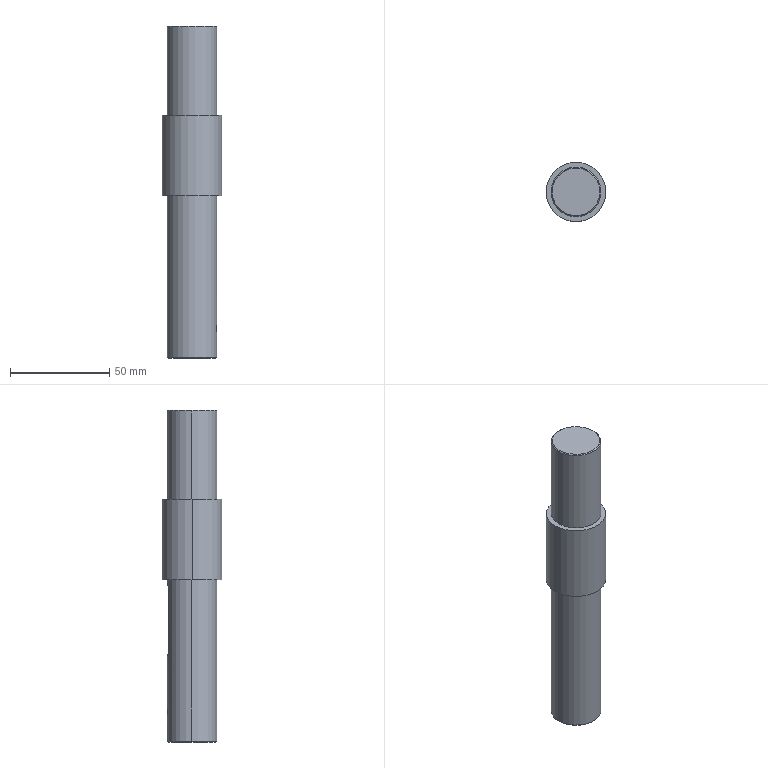Part | SolidWorks | features BaseBody 1 | 1 solid | 42 faces | box 30 x 30 x 167 mm | volume 81275 mm3 | cylinder 20 | plane 13 | cone 9 | commonest cylinder face diameters 15 x5 5 x4 25 x4 8 x3 20.5 x2 30 x2
STEP:
#1=CARTESIAN_POINT('',(0.,12.5,17.5));
#2=VERTEX_POINT('',#1);
#3=CARTESIAN_POINT('',(0.,12.5,12.5));
#4=VERTEX_POINT('',#3);
#5=CARTESIAN_POINT('',(0.,12.5,17.5));
#6=CARTESIAN_POINT('',(-0.1656,12.5,17.5));
#7=CARTESIAN_POINT('',(-0.3283,12.497,17.484));
#8=CARTESIAN_POINT('',(-0.6484,12.484,17.42));
#9=CARTESIAN_POINT('',(-0.8073,12.475,17.372));
#10=CARTESIAN_POINT('',(-1.11,12.452,17.246));
#11=CARTESIAN_POINT('',(-1.253,12.438,17.169));
#12=CARTESIAN_POINT('',(-1.525,12.407,16.988));
#13=CARTESIAN_POINT('',(-1.653,12.391,16.883));
#14=CARTESIAN_POINT('',(-1.998,12.342,16.538));
#15=CARTESIAN_POINT('',(-2.184,12.308,16.26));
#16=CARTESIAN_POINT('',(-2.371,12.273,15.809));
#17=CARTESIAN_POINT('',(-2.419,12.264,15.651));
#18=CARTESIAN_POINT('',(-2.484,12.251,15.328));
#19=CARTESIAN_POINT('',(-2.5,12.247,15.166));
#20=CARTESIAN_POINT('',(-2.5,12.247,14.839));
#21=CARTESIAN_POINT('',(-2.484,12.251,14.672));
#22=CARTESIAN_POINT('',(-2.42,12.264,14.352));
#23=CARTESIAN_POINT('',(-2.373,12.273,14.196));
#24=CARTESIAN_POINT('',(-2.247,12.297,13.892));
#25=CARTESIAN_POINT('',(-2.169,12.311,13.747));
#26=CARTESIAN_POINT('',(-1.989,12.341,13.476));
#27=CARTESIAN_POINT('',(-1.885,12.358,13.349));
#28=CARTESIAN_POINT('',(-1.653,12.391,13.117));
#29=CARTESIAN_POINT('',(-1.527,12.407,13.014));
#30=CARTESIAN_POINT('',(-1.257,12.437,12.833));
#31=CARTESIAN_POINT('',(-1.11,12.452,12.754));
#32=CARTESIAN_POINT('',(-0.8083,12.475,12.629));
#33=CARTESIAN_POINT('',(-0.6526,12.484,12.581));
#34=CARTESIAN_POINT('',(-0.3314,12.497,12.517));
#35=CARTESIAN_POINT('',(-0.1656,12.5,12.5));
#36=CARTESIAN_POINT('',(0.,12.5,12.5));
#37=B_SPLINE_CURVE_WITH_KNOTS('',3,(#5,#6,#7,#8,#9,#10,#11,#12,#13,#14,#15,#16,#17,#18,#19,#20,#21,#22,#23,#24,#25,#26,#27,#28,#29,#30,#31,#32,#33,#34,#35,#36),.UNSPECIFIED.,.F.,.F.,(4,2,2,2,2,2,2,2,2,2,2,2,2,2,2,4),(0.007834,0.008323,0.008813,0.009303,0.009792,0.01077,0.01126,0.01175,0.01224,0.01273,0.01322,0.01371,0.0142,0.01469,0.01518,0.01567),.UNSPECIFIED.);
#38=EDGE_CURVE('',#2,#4,#37,.T.);
#39=ORIENTED_EDGE('',*,*,#38,.T.);
#40=CARTESIAN_POINT('',(0.,12.5,12.5));
#41=CARTESIAN_POINT('',(0.1656,12.5,12.5));
#42=CARTESIAN_POINT('',(0.3283,12.497,12.516));
#43=CARTESIAN_POINT('',(0.6484,12.484,12.58));
#44=CARTESIAN_POINT('',(0.8073,12.475,12.628));
#45=CARTESIAN_POINT('',(1.11,12.452,12.754));
#46=CARTESIAN_POINT('',(1.253,12.438,12.831));
#47=CARTESIAN_POINT('',(1.525,12.407,13.012));
#48=CARTESIAN_POINT('',(1.653,12.391,13.117));
#49=CARTESIAN_POINT('',(1.998,12.342,13.462));
#50=CARTESIAN_POINT('',(2.184,12.308,13.74));
#51=CARTESIAN_POINT('',(2.371,12.273,14.191));
#52=CARTESIAN_POINT('',(2.419,12.264,14.349));
#53=CARTESIAN_POINT('',(2.484,12.251,14.672));
#54=CARTESIAN_POINT('',(2.5,12.247,14.834));
#55=CARTESIAN_POINT('',(2.5,12.247,15.161));
#56=CARTESIAN_POINT('',(2.484,12.251,15.328));
#57=CARTESIAN_POINT('',(2.42,12.264,15.648));
#58=CARTESIAN_POINT('',(2.373,12.273,15.804));
#59=CARTESIAN_POINT('',(2.247,12.297,16.108));
#60=CARTESIAN_POINT('',(2.169,12.311,16.253));
#61=CARTESIAN_POINT('',(1.989,12.341,16.524));
#62=CARTESIAN_POINT('',(1.885,12.358,16.651));
#63=CARTESIAN_POINT('',(1.653,12.391,16.883));
#64=CARTESIAN_POINT('',(1.527,12.407,16.986));
#65=CARTESIAN_POINT('',(1.257,12.437,17.167));
#66=CARTESIAN_POINT('',(1.11,12.452,17.246));
#67=CARTESIAN_POINT('',(0.8083,12.475,17.371));
#68=CARTESIAN_POINT('',(0.6526,12.484,17.419));
#69=CARTESIAN_POINT('',(0.3314,12.497,17.483));
#70=CARTESIAN_POINT('',(0.1656,12.5,17.5));
#71=CARTESIAN_POINT('',(0.,12.5,17.5));
#72=B_SPLINE_CURVE_WITH_KNOTS('',3,(#40,#41,#42,#43,#44,#45,#46,#47,#48,#49,#50,#51,#52,#53,#54,#55,#56,#57,#58,#59,#60,#61,#62,#63,#64,#65,#66,#67,#68,#69,#70,#71),.UNSPECIFIED.,.F.,.F.,(4,2,2,2,2,2,2,2,2,2,2,2,2,2,2,4),(0.,0.0004896,0.0009792,0.001469,0.001958,0.002938,0.003427,0.003917,0.004407,0.004896,0.005386,0.005875,0.006365,0.006855,0.007344,0.007834),.UNSPECIFIED.);
#73=EDGE_CURVE('',#4,#2,#72,.T.);
#74=ORIENTED_EDGE('',*,*,#73,.T.);
#75=EDGE_LOOP('',(#39,#74));
#76=FACE_BOUND('',#75,.T.);
#77=CARTESIAN_POINT('',(4.,11.843,46.5));
#78=VERTEX_POINT('',#77);
#79=CARTESIAN_POINT('',(4.,11.843,76.5));
#80=VERTEX_POINT('',#79);
#81=CARTESIAN_POINT('',(4.,11.843,167.));
#82=DIRECTION('',(0.,0.,1.));
#83=VECTOR('',#82,1000.);
#84=LINE('',#81,#83);
#85=EDGE_CURVE('',#78,#80,#84,.T.);
#86=ORIENTED_EDGE('',*,*,#85,.T.);
#87=CARTESIAN_POINT('',(0.,12.5,80.5));
#88=VERTEX_POINT('',#87);
#89=CARTESIAN_POINT('',(4.,11.843,76.5));
#90=CARTESIAN_POINT('',(4.,11.843,76.766));
#91=CARTESIAN_POINT('',(3.974,11.852,77.027));
#92=CARTESIAN_POINT('',(3.871,11.886,77.54));
#93=CARTESIAN_POINT('',(3.794,11.911,77.795));
#94=CARTESIAN_POINT('',(3.592,11.973,78.279));
#95=CARTESIAN_POINT('',(3.47,12.01,78.507));
#96=CARTESIAN_POINT('',(3.18,12.09,78.941));
#97=CARTESIAN_POINT('',(3.012,12.133,79.144));
#98=CARTESIAN_POINT('',(2.646,12.218,79.511));
#99=CARTESIAN_POINT('',(2.446,12.26,79.676));
#100=CARTESIAN_POINT('',(2.01,12.339,79.968));
#101=CARTESIAN_POINT('',(1.78,12.375,80.091));
#102=CARTESIAN_POINT('',(1.3,12.435,80.292));
#103=CARTESIAN_POINT('',(1.047,12.459,80.37));
#104=CARTESIAN_POINT('',(0.5285,12.492,80.474));
#105=CARTESIAN_POINT('',(0.266,12.5,80.5));
#106=CARTESIAN_POINT('',(0.,12.5,80.5));
#107=B_SPLINE_CURVE_WITH_KNOTS('',3,(#89,#90,#91,#92,#93,#94,#95,#96,#97,#98,#99,#100,#101,#102,#103,#104,#105,#106),.UNSPECIFIED.,.F.,.F.,(4,2,2,2,2,2,2,2,4),(-0.00629,-0.005504,-0.004718,-0.003932,-0.003145,-0.002359,-0.001573,-0.0007863,0.),.UNSPECIFIED.);
#108=EDGE_CURVE('',#80,#88,#107,.T.);
#109=ORIENTED_EDGE('',*,*,#108,.T.);
#110=CARTESIAN_POINT('',(-4.,11.843,76.5));
#111=VERTEX_POINT('',#110);
#112=CARTESIAN_POINT('',(0.,12.5,80.5));
#113=CARTESIAN_POINT('',(-0.266,12.5,80.5));
#114=CARTESIAN_POINT('',(-0.5272,12.492,80.474));
#115=CARTESIAN_POINT('',(-1.041,12.459,80.371));
#116=CARTESIAN_POINT('',(-1.296,12.435,80.293));
#117=CARTESIAN_POINT('',(-1.779,12.375,80.092));
#118=CARTESIAN_POINT('',(-2.008,12.34,79.969));
#119=CARTESIAN_POINT('',(-2.441,12.261,79.679));
#120=CARTESIAN_POINT('',(-2.645,12.218,79.512));
#121=CARTESIAN_POINT('',(-3.011,12.133,79.146));
#122=CARTESIAN_POINT('',(-3.176,12.091,78.946));
#123=CARTESIAN_POINT('',(-3.469,12.01,78.509));
#124=CARTESIAN_POINT('',(-3.592,11.973,78.28));
#125=CARTESIAN_POINT('',(-3.792,11.911,77.8));
#126=CARTESIAN_POINT('',(-3.87,11.886,77.546));
#127=CARTESIAN_POINT('',(-3.974,11.852,77.028));
#128=CARTESIAN_POINT('',(-4.,11.843,76.766));
#129=CARTESIAN_POINT('',(-4.,11.843,76.5));
#130=B_SPLINE_CURVE_WITH_KNOTS('',3,(#112,#113,#114,#115,#116,#117,#118,#119,#120,#121,#122,#123,#124,#125,#126,#127,#128,#129),.UNSPECIFIED.,.F.,.F.,(4,2,2,2,2,2,2,2,4),(0.,0.0007863,0.001573,0.002359,0.003145,0.003932,0.004718,0.005504,0.00629),.UNSPECIFIED.);
#131=EDGE_CURVE('',#88,#111,#130,.T.);
#132=ORIENTED_EDGE('',*,*,#131,.T.);
#133=CARTESIAN_POINT('',(-4.,11.843,46.5));
#134=VERTEX_POINT('',#133);
#135=CARTESIAN_POINT('',(-4.,11.843,167.));
#136=DIRECTION('',(0.,0.,-1.));
#137=VECTOR('',#136,1000.);
#138=LINE('',#135,#137);
#139=EDGE_CURVE('',#111,#134,#138,.T.);
#140=ORIENTED_EDGE('',*,*,#139,.T.);
#141=CARTESIAN_POINT('',(-4.,11.843,46.5));
#142=CARTESIAN_POINT('',(-4.,11.843,46.234));
#143=CARTESIAN_POINT('',(-3.974,11.852,45.973));
#144=CARTESIAN_POINT('',(-3.871,11.886,45.459));
#145=CARTESIAN_POINT('',(-3.793,11.911,45.204));
#146=CARTESIAN_POINT('',(-3.592,11.973,44.721));
#147=CARTESIAN_POINT('',(-3.469,12.01,44.492));
#148=CARTESIAN_POINT('',(-3.179,12.09,44.059));
#149=CARTESIAN_POINT('',(-3.012,12.133,43.855));
#150=CARTESIAN_POINT('',(-2.646,12.218,43.489));
#151=CARTESIAN_POINT('',(-2.445,12.26,43.324));
#152=CARTESIAN_POINT('',(-2.009,12.34,43.031));
#153=CARTESIAN_POINT('',(-1.779,12.375,42.908));
#154=CARTESIAN_POINT('',(-1.299,12.435,42.708));
#155=CARTESIAN_POINT('',(-1.045,12.459,42.63));
#156=CARTESIAN_POINT('',(-0.5276,12.492,42.526));
#157=CARTESIAN_POINT('',(-0.2669,12.5,42.5));
#158=CARTESIAN_POINT('',(0.2587,12.5,42.5));
#159=CARTESIAN_POINT('',(0.5256,12.492,42.526));
#160=CARTESIAN_POINT('',(1.04,12.459,42.629));
#161=CARTESIAN_POINT('',(1.29,12.436,42.705));
#162=CARTESIAN_POINT('',(1.777,12.375,42.907));
#163=CARTESIAN_POINT('',(2.008,12.34,43.031));
#164=CARTESIAN_POINT('',(2.44,12.262,43.32));
#165=CARTESIAN_POINT('',(2.643,12.219,43.487));
#166=CARTESIAN_POINT('',(3.012,12.133,43.855));
#167=CARTESIAN_POINT('',(3.176,12.091,44.055));
#168=CARTESIAN_POINT('',(3.466,12.011,44.487));
#169=CARTESIAN_POINT('',(3.592,11.973,44.72));
#170=CARTESIAN_POINT('',(3.792,11.911,45.202));
#171=CARTESIAN_POINT('',(3.869,11.886,45.451));
#172=CARTESIAN_POINT('',(3.973,11.852,45.968));
#173=CARTESIAN_POINT('',(4.,11.843,46.234));
#174=CARTESIAN_POINT('',(4.,11.843,46.5));
#175=B_SPLINE_CURVE_WITH_KNOTS('',3,(#141,#142,#143,#144,#145,#146,#147,#148,#149,#150,#151,#152,#153,#154,#155,#156,#157,#158,#159,#160,#161,#162,#163,#164,#165,#166,#167,#168,#169,#170,#171,#172,#173,#174),.UNSPECIFIED.,.F.,.F.,(4,2,2,2,2,2,2,2,2,2,2,2,2,2,2,2,4),(0.,0.0007865,0.001573,0.00236,0.003146,0.003933,0.004719,0.005506,0.006292,0.007079,0.007865,0.008652,0.009438,0.01022,0.01101,0.0118,0.01258),.UNSPECIFIED.);
#176=EDGE_CURVE('',#134,#78,#175,.T.);
#177=ORIENTED_EDGE('',*,*,#176,.T.);
#178=EDGE_LOOP('',(#86,#109,#132,#140,#177));
#179=FACE_BOUND('',#178,.T.);
#180=CARTESIAN_POINT('',(-12.5,0.,81.5));
#181=VERTEX_POINT('',#180);
#182=CARTESIAN_POINT('',(12.5,0.,81.5));
#183=VERTEX_POINT('',#182);
#184=CARTESIAN_POINT('',(0.,0.,81.5));
#185=DIRECTION('',(0.,0.,-1.));
#186=DIRECTION('',(-1.,0.,0.));
#187=AXIS2_PLACEMENT_3D('',#184,#185,#186);
#188=CIRCLE('',#187,12.5);
#189=EDGE_CURVE('',#181,#183,#188,.T.);
#190=ORIENTED_EDGE('',*,*,#189,.T.);
#191=CARTESIAN_POINT('',(12.5,0.,17.5));
#192=VERTEX_POINT('',#191);
#193=CARTESIAN_POINT('',(12.5,0.,167.));
#194=DIRECTION('',(0.,0.,-1.));
#195=VECTOR('',#194,1000.);
#196=LINE('',#193,#195);
#197=EDGE_CURVE('',#183,#192,#196,.T.);
#198=ORIENTED_EDGE('',*,*,#197,.T.);
#199=CARTESIAN_POINT('',(12.5,0.,12.5));
#200=VERTEX_POINT('',#199);
#201=CARTESIAN_POINT('',(12.5,0.,17.5));
#202=CARTESIAN_POINT('',(12.5,0.1656,17.5));
#203=CARTESIAN_POINT('',(12.497,0.3283,17.484));
#204=CARTESIAN_POINT('',(12.484,0.6484,17.42));
#205=CARTESIAN_POINT('',(12.475,0.8073,17.372));
#206=CARTESIAN_POINT('',(12.452,1.11,17.246));
#207=CARTESIAN_POINT('',(12.438,1.253,17.169));
#208=CARTESIAN_POINT('',(12.407,1.525,16.988));
#209=CARTESIAN_POINT('',(12.391,1.653,16.883));
#210=CARTESIAN_POINT('',(12.342,1.998,16.538));
#211=CARTESIAN_POINT('',(12.308,2.184,16.26));
#212=CARTESIAN_POINT('',(12.273,2.371,15.809));
#213=CARTESIAN_POINT('',(12.264,2.419,15.651));
#214=CARTESIAN_POINT('',(12.251,2.484,15.328));
#215=CARTESIAN_POINT('',(12.247,2.5,15.166));
#216=CARTESIAN_POINT('',(12.247,2.5,14.839));
#217=CARTESIAN_POINT('',(12.251,2.484,14.672));
#218=CARTESIAN_POINT('',(12.264,2.42,14.352));
#219=CARTESIAN_POINT('',(12.273,2.373,14.196));
#220=CARTESIAN_POINT('',(12.297,2.247,13.892));
#221=CARTESIAN_POINT('',(12.311,2.169,13.747));
#222=CARTESIAN_POINT('',(12.341,1.989,13.476));
#223=CARTESIAN_POINT('',(12.358,1.885,13.349));
#224=CARTESIAN_POINT('',(12.391,1.653,13.117));
#225=CARTESIAN_POINT('',(12.407,1.527,13.014));
#226=CARTESIAN_POINT('',(12.437,1.257,12.833));
#227=CARTESIAN_POINT('',(12.452,1.11,12.754));
#228=CARTESIAN_POINT('',(12.475,0.8083,12.629));
#229=CARTESIAN_POINT('',(12.484,0.6526,12.581));
#230=CARTESIAN_POINT('',(12.497,0.3314,12.517));
#231=CARTESIAN_POINT('',(12.5,0.1656,12.5));
#232=CARTESIAN_POINT('',(12.5,0.,12.5));
#233=B_SPLINE_CURVE_WITH_KNOTS('',3,(#201,#202,#203,#204,#205,#206,#207,#208,#209,#210,#211,#212,#213,#214,#215,#216,#217,#218,#219,#220,#221,#222,#223,#224,#225,#226,#227,#228,#229,#230,#231,#232),.UNSPECIFIED.,.F.,.F.,(4,2,2,2,2,2,2,2,2,2,2,2,2,2,2,4),(0.007834,0.008323,0.008813,0.009303,0.009792,0.01077,0.01126,0.01175,0.01224,0.01273,0.01322,0.01371,0.0142,0.01469,0.01518,0.01567),.UNSPECIFIED.);
#234=EDGE_CURVE('',#192,#200,#233,.T.);
#235=ORIENTED_EDGE('',*,*,#234,.T.);
#236=CARTESIAN_POINT('',(12.5,0.,0.5));
#237=VERTEX_POINT('',#236);
#238=CARTESIAN_POINT('',(12.5,0.,167.));
#239=DIRECTION('',(0.,0.,-1.));
#240=VECTOR('',#239,1000.);
#241=LINE('',#238,#240);
#242=EDGE_CURVE('',#200,#237,#241,.T.);
#243=ORIENTED_EDGE('',*,*,#242,.T.);
#244=CARTESIAN_POINT('',(-12.5,0.,0.5));
#245=VERTEX_POINT('',#244);
#246=CARTESIAN_POINT('',(0.,0.,0.5));
#247=DIRECTION('',(0.,0.,1.));
#248=DIRECTION('',(-1.,0.,0.));
#249=AXIS2_PLACEMENT_3D('',#246,#247,#248);
#250=CIRCLE('',#249,12.5);
#251=EDGE_CURVE('',#237,#245,#250,.T.);
#252=ORIENTED_EDGE('',*,*,#251,.T.);
#253=CARTESIAN_POINT('',(-12.5,0.,167.));
#254=DIRECTION('',(0.,0.,-1.));
#255=VECTOR('',#254,1000.);
#256=LINE('',#253,#255);
#257=EDGE_CURVE('',#181,#245,#256,.T.);
#258=ORIENTED_EDGE('',*,*,#257,.F.);
#259=EDGE_LOOP('',(#190,#198,#235,#243,#252,#258));
#260=FACE_OUTER_BOUND('',#259,.T.);
#261=CARTESIAN_POINT('',(0.,0.,167.));
#262=DIRECTION('',(0.,0.,-1.));
#263=DIRECTION('',(-1.,0.,0.));
#264=AXIS2_PLACEMENT_3D('',#261,#262,#263);
#265=CYLINDRICAL_SURFACE('',#264,12.5);
#266=ADVANCED_FACE('',(#76,#179,#260),#265,.T.);
#267=CARTESIAN_POINT('',(7.5,0.,17.5));
#268=VERTEX_POINT('',#267);
#269=CARTESIAN_POINT('',(7.5,0.,12.5));
#270=VERTEX_POINT('',#269);
#271=CARTESIAN_POINT('',(7.5,0.,17.5));
#272=CARTESIAN_POINT('',(7.5,-0.1664,17.5));
#273=CARTESIAN_POINT('',(7.494,-0.3298,17.484));
#274=CARTESIAN_POINT('',(7.473,-0.6509,17.419));
#275=CARTESIAN_POINT('',(7.458,-0.8103,17.371));
#276=CARTESIAN_POINT('',(7.419,-1.112,17.245));
#277=CARTESIAN_POINT('',(7.395,-1.256,17.168));
#278=CARTESIAN_POINT('',(7.344,-1.526,16.987));
#279=CARTESIAN_POINT('',(7.316,-1.654,16.882));
#280=CARTESIAN_POINT('',(7.233,-1.997,16.539));
#281=CARTESIAN_POINT('',(7.177,-2.182,16.262));
#282=CARTESIAN_POINT('',(7.116,-2.37,15.812));
#283=CARTESIAN_POINT('',(7.099,-2.419,15.653));
#284=CARTESIAN_POINT('',(7.077,-2.484,15.33));
#285=CARTESIAN_POINT('',(7.071,-2.5,15.167));
#286=CARTESIAN_POINT('',(7.071,-2.5,14.838));
#287=CARTESIAN_POINT('',(7.077,-2.484,14.671));
#288=CARTESIAN_POINT('',(7.099,-2.42,14.35));
#289=CARTESIAN_POINT('',(7.115,-2.372,14.193));
#290=CARTESIAN_POINT('',(7.156,-2.246,13.889));
#291=CARTESIAN_POINT('',(7.18,-2.168,13.745));
#292=CARTESIAN_POINT('',(7.232,-1.988,13.475));
#293=CARTESIAN_POINT('',(7.261,-1.884,13.348));
#294=CARTESIAN_POINT('',(7.316,-1.654,13.118));
#295=CARTESIAN_POINT('',(7.344,-1.529,13.015));
#296=CARTESIAN_POINT('',(7.395,-1.259,12.834));
#297=CARTESIAN_POINT('',(7.419,-1.113,12.755));
#298=CARTESIAN_POINT('',(7.457,-0.812,12.63));
#299=CARTESIAN_POINT('',(7.473,-0.6561,12.582));
#300=CARTESIAN_POINT('',(7.494,-0.3326,12.517));
#301=CARTESIAN_POINT('',(7.5,-0.1664,12.5));
#302=CARTESIAN_POINT('',(7.5,0.,12.5));
#303=B_SPLINE_CURVE_WITH_KNOTS('',3,(#271,#272,#273,#274,#275,#276,#277,#278,#279,#280,#281,#282,#283,#284,#285,#286,#287,#288,#289,#290,#291,#292,#293,#294,#295,#296,#297,#298,#299,#300,#301,#302),.UNSPECIFIED.,.F.,.F.,(4,2,2,2,2,2,2,2,2,2,2,2,2,2,2,4),(0.,0.0004919,0.0009837,0.001476,0.001967,0.002951,0.003443,0.003935,0.004427,0.004919,0.005411,0.005902,0.006394,0.006886,0.007378,0.00787),.UNSPECIFIED.);
#304=EDGE_CURVE('',#268,#270,#303,.T.);
#305=ORIENTED_EDGE('',*,*,#304,.F.);
#306=CARTESIAN_POINT('',(12.5,0.,17.5));
#307=DIRECTION('',(1.,0.,0.));
#308=VECTOR('',#307,1000.);
#309=LINE('',#306,#308);
#310=EDGE_CURVE('',#268,#192,#309,.T.);
#311=ORIENTED_EDGE('',*,*,#310,.T.);
#312=CARTESIAN_POINT('',(12.5,0.,12.5));
#313=CARTESIAN_POINT('',(12.5,-0.1656,12.5));
#314=CARTESIAN_POINT('',(12.497,-0.3283,12.516));
#315=CARTESIAN_POINT('',(12.484,-0.6484,12.58));
#316=CARTESIAN_POINT('',(12.475,-0.8073,12.628));
#317=CARTESIAN_POINT('',(12.452,-1.11,12.754));
#318=CARTESIAN_POINT('',(12.438,-1.253,12.831));
#319=CARTESIAN_POINT('',(12.407,-1.525,13.012));
#320=CARTESIAN_POINT('',(12.391,-1.653,13.117));
#321=CARTESIAN_POINT('',(12.342,-1.998,13.462));
#322=CARTESIAN_POINT('',(12.308,-2.184,13.74));
#323=CARTESIAN_POINT('',(12.273,-2.371,14.191));
#324=CARTESIAN_POINT('',(12.264,-2.419,14.349));
#325=CARTESIAN_POINT('',(12.251,-2.484,14.672));
#326=CARTESIAN_POINT('',(12.247,-2.5,14.834));
#327=CARTESIAN_POINT('',(12.247,-2.5,15.161));
#328=CARTESIAN_POINT('',(12.251,-2.484,15.328));
#329=CARTESIAN_POINT('',(12.264,-2.42,15.648));
#330=CARTESIAN_POINT('',(12.273,-2.373,15.804));
#331=CARTESIAN_POINT('',(12.297,-2.247,16.108));
#332=CARTESIAN_POINT('',(12.311,-2.169,16.253));
#333=CARTESIAN_POINT('',(12.341,-1.989,16.524));
#334=CARTESIAN_POINT('',(12.358,-1.885,16.651));
#335=CARTESIAN_POINT('',(12.391,-1.653,16.883));
#336=CARTESIAN_POINT('',(12.407,-1.527,16.986));
#337=CARTESIAN_POINT('',(12.437,-1.257,17.167));
#338=CARTESIAN_POINT('',(12.452,-1.11,17.246));
#339=CARTESIAN_POINT('',(12.475,-0.8083,17.371));
#340=CARTESIAN_POINT('',(12.484,-0.6526,17.419));
#341=CARTESIAN_POINT('',(12.497,-0.3314,17.483));
#342=CARTESIAN_POINT('',(12.5,-0.1656,17.5));
#343=CARTESIAN_POINT('',(12.5,0.,17.5));
#344=B_SPLINE_CURVE_WITH_KNOTS('',3,(#312,#313,#314,#315,#316,#317,#318,#319,#320,#321,#322,#323,#324,#325,#326,#327,#328,#329,#330,#331,#332,#333,#334,#335,#336,#337,#338,#339,#340,#341,#342,#343),.UNSPECIFIED.,.F.,.F.,(4,2,2,2,2,2,2,2,2,2,2,2,2,2,2,4),(0.,0.0004896,0.0009792,0.001469,0.001958,0.002938,0.003427,0.003917,0.004407,0.004896,0.005386,0.005875,0.006365,0.006855,0.007344,0.007834),.UNSPECIFIED.);
#345=EDGE_CURVE('',#200,#192,#344,.T.);
#346=ORIENTED_EDGE('',*,*,#345,.F.);
#347=CARTESIAN_POINT('',(12.5,0.,12.5));
#348=DIRECTION('',(1.,0.,0.));
#349=VECTOR('',#348,1000.);
#350=LINE('',#347,#349);
#351=EDGE_CURVE('',#270,#200,#350,.T.);
#352=ORIENTED_EDGE('',*,*,#351,.F.);
#353=EDGE_LOOP('',(#305,#311,#346,#352));
#354=FACE_OUTER_BOUND('',#353,.T.);
#355=CARTESIAN_POINT('',(12.5,0.,15.));
#356=DIRECTION('',(1.,0.,0.));
#357=DIRECTION('',(0.,0.,-1.));
#358=AXIS2_PLACEMENT_3D('',#355,#356,#357);
#359=CYLINDRICAL_SURFACE('',#358,2.5);
#360=ADVANCED_FACE('',(#354),#359,.F.);
#361=CARTESIAN_POINT('',(12.,0.,0.));
#362=VERTEX_POINT('',#361);
#363=CARTESIAN_POINT('',(-12.,0.,0.));
#364=VERTEX_POINT('',#363);
#365=CARTESIAN_POINT('',(0.,0.,0.));
#366=DIRECTION('',(0.,0.,1.));
#367=DIRECTION('',(1.,0.,0.));
#368=AXIS2_PLACEMENT_3D('',#365,#366,#367);
#369=CIRCLE('',#368,12.);
#370=EDGE_CURVE('',#362,#364,#369,.T.);
#371=ORIENTED_EDGE('',*,*,#370,.T.);
#372=CARTESIAN_POINT('',(-12.5,0.,0.5));
#373=DIRECTION('',(-0.7071,0.,0.7071));
#374=VECTOR('',#373,1000.);
#375=LINE('',#372,#374);
#376=EDGE_CURVE('',#364,#245,#375,.T.);
#377=ORIENTED_EDGE('',*,*,#376,.T.);
#378=ORIENTED_EDGE('',*,*,#251,.F.);
#379=CARTESIAN_POINT('',(12.5,0.,0.5));
#380=DIRECTION('',(0.7071,0.,0.7071));
#381=VECTOR('',#380,1000.);
#382=LINE('',#379,#381);
#383=EDGE_CURVE('',#362,#237,#382,.T.);
#384=ORIENTED_EDGE('',*,*,#383,.F.);
#385=EDGE_LOOP('',(#371,#377,#378,#384));
#386=FACE_OUTER_BOUND('',#385,.T.);
#387=CARTESIAN_POINT('',(0.,0.,0.5));
#388=DIRECTION('',(0.,0.,1.));
#389=DIRECTION('',(1.,0.,0.));
#390=AXIS2_PLACEMENT_3D('',#387,#388,#389);
#391=CONICAL_SURFACE('',#390,12.5,0.7854);
#392=ADVANCED_FACE('',(#386),#391,.T.);
#393=CARTESIAN_POINT('',(7.5,0.,35.));
#394=VERTEX_POINT('',#393);
#395=CARTESIAN_POINT('',(-7.5,0.,35.));
#396=VERTEX_POINT('',#395);
#397=CARTESIAN_POINT('',(0.,0.,35.));
#398=DIRECTION('',(0.,0.,-1.));
#399=DIRECTION('',(-1.,0.,0.));
#400=AXIS2_PLACEMENT_3D('',#397,#398,#399);
#401=CIRCLE('',#400,7.5);
#402=EDGE_CURVE('',#394,#396,#401,.T.);
#403=ORIENTED_EDGE('',*,*,#402,.F.);
#404=CARTESIAN_POINT('',(7.5,0.,0.));
#405=DIRECTION('',(0.,0.,-1.));
#406=VECTOR('',#405,1000.);
#407=LINE('',#404,#406);
#408=EDGE_CURVE('',#394,#268,#407,.T.);
#409=ORIENTED_EDGE('',*,*,#408,.T.);
#410=ORIENTED_EDGE('',*,*,#304,.T.);
#411=CARTESIAN_POINT('',(7.5,0.,0.5));
#412=VERTEX_POINT('',#411);
#413=CARTESIAN_POINT('',(7.5,0.,0.));
#414=DIRECTION('',(0.,0.,-1.));
#415=VECTOR('',#414,1000.);
#416=LINE('',#413,#415);
#417=EDGE_CURVE('',#270,#412,#416,.T.);
#418=ORIENTED_EDGE('',*,*,#417,.T.);
#419=CARTESIAN_POINT('',(-7.5,0.,0.5));
#420=VERTEX_POINT('',#419);
#421=CARTESIAN_POINT('',(0.,0.,0.5));
#422=DIRECTION('',(0.,0.,1.));
#423=DIRECTION('',(-1.,0.,0.));
#424=AXIS2_PLACEMENT_3D('',#421,#422,#423);
#425=CIRCLE('',#424,7.5);
#426=EDGE_CURVE('',#420,#412,#425,.T.);
#427=ORIENTED_EDGE('',*,*,#426,.F.);
#428=CARTESIAN_POINT('',(-7.5,0.,0.));
#429=DIRECTION('',(0.,0.,-1.));
#430=VECTOR('',#429,1000.);
#431=LINE('',#428,#430);
#432=EDGE_CURVE('',#396,#420,#431,.T.);
#433=ORIENTED_EDGE('',*,*,#432,.F.);
#434=EDGE_LOOP('',(#403,#409,#410,#418,#427,#433));
#435=FACE_OUTER_BOUND('',#434,.T.);
#436=CARTESIAN_POINT('',(0.,0.,0.));
#437=DIRECTION('',(0.,0.,-1.));
#438=DIRECTION('',(-1.,0.,0.));
#439=AXIS2_PLACEMENT_3D('',#436,#437,#438);
#440=CYLINDRICAL_SURFACE('',#439,7.5);
#441=ADVANCED_FACE('',(#435),#440,.F.);
#442=CARTESIAN_POINT('',(-2.5,7.071,35.));
#443=VERTEX_POINT('',#442);
#444=CARTESIAN_POINT('',(0.,0.,35.));
#445=DIRECTION('',(0.,0.,-1.));
#446=DIRECTION('',(-1.,0.,0.));
#447=AXIS2_PLACEMENT_3D('',#444,#445,#446);
#448=CIRCLE('',#447,7.5);
#449=EDGE_CURVE('',#396,#443,#448,.T.);
#450=ORIENTED_EDGE('',*,*,#449,.F.);
#451=ORIENTED_EDGE('',*,*,#432,.T.);
#452=CARTESIAN_POINT('',(-2.5,7.071,0.5));
#453=VERTEX_POINT('',#452);
#454=CARTESIAN_POINT('',(0.,0.,0.5));
#455=DIRECTION('',(0.,0.,1.));
#456=DIRECTION('',(-1.,0.,0.));
#457=AXIS2_PLACEMENT_3D('',#454,#455,#456);
#458=CIRCLE('',#457,7.5);
#459=EDGE_CURVE('',#453,#420,#458,.T.);
#460=ORIENTED_EDGE('',*,*,#459,.F.);
#461=CARTESIAN_POINT('',(-2.5,7.071,0.));
#462=DIRECTION('',(0.,0.,-1.));
#463=VECTOR('',#462,1000.);
#464=LINE('',#461,#463);
#465=EDGE_CURVE('',#443,#453,#464,.T.);
#466=ORIENTED_EDGE('',*,*,#465,.F.);
#467=EDGE_LOOP('',(#450,#451,#460,#466));
#468=FACE_OUTER_BOUND('',#467,.T.);
#469=CARTESIAN_POINT('',(0.,0.,0.));
#470=DIRECTION('',(0.,0.,-1.));
#471=DIRECTION('',(-1.,0.,0.));
#472=AXIS2_PLACEMENT_3D('',#469,#470,#471);
#473=CYLINDRICAL_SURFACE('',#472,7.5);
#474=ADVANCED_FACE('',(#468),#473,.F.);
#475=CARTESIAN_POINT('',(0.,9.8,12.5));
#476=VERTEX_POINT('',#475);
#477=CARTESIAN_POINT('',(-2.5,9.8,15.));
#478=VERTEX_POINT('',#477);
#479=CARTESIAN_POINT('',(0.,9.8,15.));
#480=DIRECTION('',(0.,1.,0.));
#481=DIRECTION('',(0.,0.,1.));
#482=AXIS2_PLACEMENT_3D('',#479,#480,#481);
#483=CIRCLE('',#482,2.5);
#484=EDGE_CURVE('',#476,#478,#483,.T.);
#485=ORIENTED_EDGE('',*,*,#484,.F.);
#486=CARTESIAN_POINT('',(0.,12.5,12.5));
#487=DIRECTION('',(0.,1.,0.));
#488=VECTOR('',#487,1000.);
#489=LINE('',#486,#488);
#490=EDGE_CURVE('',#476,#4,#489,.T.);
#491=ORIENTED_EDGE('',*,*,#490,.T.);
#492=ORIENTED_EDGE('',*,*,#38,.F.);
#493=CARTESIAN_POINT('',(0.,9.8,17.5));
#494=VERTEX_POINT('',#493);
#495=CARTESIAN_POINT('',(0.,12.5,17.5));
#496=DIRECTION('',(0.,1.,0.));
#497=VECTOR('',#496,1000.);
#498=LINE('',#495,#497);
#499=EDGE_CURVE('',#494,#2,#498,.T.);
#500=ORIENTED_EDGE('',*,*,#499,.F.);
#501=CARTESIAN_POINT('',(0.,9.8,15.));
#502=DIRECTION('',(0.,1.,0.));
#503=DIRECTION('',(0.,0.,1.));
#504=AXIS2_PLACEMENT_3D('',#501,#502,#503);
#505=CIRCLE('',#504,2.5);
#506=EDGE_CURVE('',#478,#494,#505,.T.);
#507=ORIENTED_EDGE('',*,*,#506,.F.);
#508=EDGE_LOOP('',(#485,#491,#492,#500,#507));
#509=FACE_OUTER_BOUND('',#508,.T.);
#510=CARTESIAN_POINT('',(0.,12.5,15.));
#511=DIRECTION('',(0.,1.,0.));
#512=DIRECTION('',(0.,0.,1.));
#513=AXIS2_PLACEMENT_3D('',#510,#511,#512);
#514=CYLINDRICAL_SURFACE('',#513,2.5);
#515=ADVANCED_FACE('',(#509),#514,.F.);
#516=CARTESIAN_POINT('',(0.,9.2,80.5));
#517=VERTEX_POINT('',#516);
#518=CARTESIAN_POINT('',(4.,9.2,76.5));
#519=VERTEX_POINT('',#518);
#520=CARTESIAN_POINT('',(0.,9.2,76.5));
#521=DIRECTION('',(0.,1.,0.));
#522=DIRECTION('',(0.,0.,1.));
#523=AXIS2_PLACEMENT_3D('',#520,#521,#522);
#524=CIRCLE('',#523,4.);
#525=EDGE_CURVE('',#517,#519,#524,.T.);
#526=ORIENTED_EDGE('',*,*,#525,.F.);
#527=CARTESIAN_POINT('',(0.,9.2,80.5));
#528=DIRECTION('',(0.,1.,0.));
#529=VECTOR('',#528,1000.);
#530=LINE('',#527,#529);
#531=EDGE_CURVE('',#517,#88,#530,.T.);
#532=ORIENTED_EDGE('',*,*,#531,.T.);
#533=ORIENTED_EDGE('',*,*,#108,.F.);
#534=CARTESIAN_POINT('',(4.,9.2,76.5));
#535=DIRECTION('',(0.,1.,0.));
#536=VECTOR('',#535,1000.);
#537=LINE('',#534,#536);
#538=EDGE_CURVE('',#519,#80,#537,.T.);
#539=ORIENTED_EDGE('',*,*,#538,.F.);
#540=EDGE_LOOP('',(#526,#532,#533,#539));
#541=FACE_OUTER_BOUND('',#540,.T.);
#542=CARTESIAN_POINT('',(0.,9.2,76.5));
#543=DIRECTION('',(0.,1.,0.));
#544=DIRECTION('',(0.,0.,1.));
#545=AXIS2_PLACEMENT_3D('',#542,#543,#544);
#546=CYLINDRICAL_SURFACE('',#545,4.);
#547=ADVANCED_FACE('',(#541),#546,.F.);
#548=CARTESIAN_POINT('',(-15.,0.,122.));
#549=VERTEX_POINT('',#548);
#550=CARTESIAN_POINT('',(15.,0.,122.));
#551=VERTEX_POINT('',#550);
#552=CARTESIAN_POINT('',(0.,0.,122.));
#553=DIRECTION('',(0.,0.,-1.));
#554=DIRECTION('',(-1.,0.,0.));
#555=AXIS2_PLACEMENT_3D('',#552,#553,#554);
#556=CIRCLE('',#555,15.);
#557=EDGE_CURVE('',#549,#551,#556,.T.);
#558=ORIENTED_EDGE('',*,*,#557,.T.);
#559=CARTESIAN_POINT('',(15.,0.,81.5));
#560=VERTEX_POINT('',#559);
#561=CARTESIAN_POINT('',(15.,0.,164.426));
#562=DIRECTION('',(0.,0.,-1.));
#563=VECTOR('',#562,1000.);
#564=LINE('',#561,#563);
#565=EDGE_CURVE('',#551,#560,#564,.T.);
#566=ORIENTED_EDGE('',*,*,#565,.T.);
#567=CARTESIAN_POINT('',(-15.,0.,81.5));
#568=VERTEX_POINT('',#567);
#569=CARTESIAN_POINT('',(0.,0.,81.5));
#570=DIRECTION('',(0.,0.,1.));
#571=DIRECTION('',(-1.,0.,0.));
#572=AXIS2_PLACEMENT_3D('',#569,#570,#571);
#573=CIRCLE('',#572,15.);
#574=EDGE_CURVE('',#560,#568,#573,.T.);
#575=ORIENTED_EDGE('',*,*,#574,.T.);
#576=CARTESIAN_POINT('',(-15.,0.,164.426));
#577=DIRECTION('',(0.,0.,-1.));
#578=VECTOR('',#577,1000.);
#579=LINE('',#576,#578);
#580=EDGE_CURVE('',#549,#568,#579,.T.);
#581=ORIENTED_EDGE('',*,*,#580,.F.);
#582=EDGE_LOOP('',(#558,#566,#575,#581));
#583=FACE_OUTER_BOUND('',#582,.T.);
#584=CARTESIAN_POINT('',(0.,0.,164.426));
#585=DIRECTION('',(0.,0.,-1.));
#586=DIRECTION('',(-1.,0.,0.));
#587=AXIS2_PLACEMENT_3D('',#584,#585,#586);
#588=CYLINDRICAL_SURFACE('',#587,15.);
#589=ADVANCED_FACE('',(#583),#588,.T.);
#590=ORIENTED_EDGE('',*,*,#426,.T.);
#591=CARTESIAN_POINT('',(8.,0.,0.));
#592=VERTEX_POINT('',#591);
#593=CARTESIAN_POINT('',(8.,0.,0.));
#594=DIRECTION('',(0.7071,0.,-0.7071));
#595=VECTOR('',#594,1000.);
#596=LINE('',#593,#595);
#597=EDGE_CURVE('',#412,#592,#596,.T.);
#598=ORIENTED_EDGE('',*,*,#597,.T.);
#599=CARTESIAN_POINT('',(-8.,0.,0.));
#600=VERTEX_POINT('',#599);
#601=CARTESIAN_POINT('',(0.,0.,0.));
#602=DIRECTION('',(0.,0.,-1.));
#603=DIRECTION('',(-1.,0.,0.));
#604=AXIS2_PLACEMENT_3D('',#601,#602,#603);
#605=CIRCLE('',#604,8.);
#606=EDGE_CURVE('',#592,#600,#605,.T.);
#607=ORIENTED_EDGE('',*,*,#606,.T.);
#608=CARTESIAN_POINT('',(-8.,0.,0.));
#609=DIRECTION('',(-0.7071,0.,-0.7071));
#610=VECTOR('',#609,1000.);
#611=LINE('',#608,#610);
#612=EDGE_CURVE('',#420,#600,#611,.T.);
#613=ORIENTED_EDGE('',*,*,#612,.F.);
#614=EDGE_LOOP('',(#590,#598,#607,#613));
#615=FACE_OUTER_BOUND('',#614,.T.);
#616=CARTESIAN_POINT('',(0.,0.,0.));
#617=DIRECTION('',(0.,0.,-1.));
#618=DIRECTION('',(-1.,0.,0.));
#619=AXIS2_PLACEMENT_3D('',#616,#617,#618);
#620=CONICAL_SURFACE('',#619,8.,0.7854);
#621=ADVANCED_FACE('',(#615),#620,.F.);
#622=ORIENTED_EDGE('',*,*,#459,.T.);
#623=ORIENTED_EDGE('',*,*,#612,.T.);
#624=CARTESIAN_POINT('',(-2.5,7.599,0.));
#625=VERTEX_POINT('',#624);
#626=CARTESIAN_POINT('',(0.,0.,0.));
#627=DIRECTION('',(0.,0.,-1.));
#628=DIRECTION('',(-1.,0.,0.));
#629=AXIS2_PLACEMENT_3D('',#626,#627,#628);
#630=CIRCLE('',#629,8.);
#631=EDGE_CURVE('',#600,#625,#630,.T.);
#632=ORIENTED_EDGE('',*,*,#631,.T.);
#633=CARTESIAN_POINT('',(-2.5,7.599,0.));
#634=CARTESIAN_POINT('',(-2.5,7.424,0.167));
#635=CARTESIAN_POINT('',(-2.5,7.247,0.3337));
#636=CARTESIAN_POINT('',(-2.5,7.071,0.5));
#637=B_SPLINE_CURVE_WITH_KNOTS('',3,(#633,#634,#635,#636),.UNSPECIFIED.,.F.,.F.,(4,4),(0.,0.0007274),.UNSPECIFIED.);
#638=EDGE_CURVE('',#625,#453,#637,.T.);
#639=ORIENTED_EDGE('',*,*,#638,.T.);
#640=EDGE_LOOP('',(#622,#623,#632,#639));
#641=FACE_OUTER_BOUND('',#640,.T.);
#642=CARTESIAN_POINT('',(0.,0.,0.));
#643=DIRECTION('',(0.,0.,-1.));
#644=DIRECTION('',(-1.,0.,0.));
#645=AXIS2_PLACEMENT_3D('',#642,#643,#644);
#646=CONICAL_SURFACE('',#645,8.,0.7854);
#647=ADVANCED_FACE('',(#641),#646,.F.);
#648=CARTESIAN_POINT('',(10.25,0.,39.));
#649=VERTEX_POINT('',#648);
#650=CARTESIAN_POINT('',(-10.25,0.,39.));
#651=VERTEX_POINT('',#650);
#652=CARTESIAN_POINT('',(0.,0.,39.));
#653=DIRECTION('',(0.,0.,-1.));
#654=DIRECTION('',(-1.,0.,0.));
#655=AXIS2_PLACEMENT_3D('',#652,#653,#654);
#656=CIRCLE('',#655,10.25);
#657=EDGE_CURVE('',#649,#651,#656,.T.);
#658=ORIENTED_EDGE('',*,*,#657,.F.);
#659=CARTESIAN_POINT('',(10.25,0.,35.));
#660=VERTEX_POINT('',#659);
#661=CARTESIAN_POINT('',(10.25,0.,39.));
#662=DIRECTION('',(0.,0.,-1.));
#663=VECTOR('',#662,1000.);
#664=LINE('',#661,#663);
#665=EDGE_CURVE('',#649,#660,#664,.T.);
#666=ORIENTED_EDGE('',*,*,#665,.T.);
#667=CARTESIAN_POINT('',(-10.25,0.,35.));
#668=VERTEX_POINT('',#667);
#669=CARTESIAN_POINT('',(0.,0.,35.));
#670=DIRECTION('',(0.,0.,-1.));
#671=DIRECTION('',(-1.,0.,0.));
#672=AXIS2_PLACEMENT_3D('',#669,#670,#671);
#673=CIRCLE('',#672,10.25);
#674=EDGE_CURVE('',#660,#668,#673,.T.);
#675=ORIENTED_EDGE('',*,*,#674,.T.);
#676=CARTESIAN_POINT('',(-10.25,0.,39.));
#677=DIRECTION('',(0.,0.,-1.));
#678=VECTOR('',#677,1000.);
#679=LINE('',#676,#678);
#680=EDGE_CURVE('',#651,#668,#679,.T.);
#681=ORIENTED_EDGE('',*,*,#680,.F.);
#682=EDGE_LOOP('',(#658,#666,#675,#681));
#683=FACE_OUTER_BOUND('',#682,.T.);
#684=CARTESIAN_POINT('',(0.,0.,39.));
#685=DIRECTION('',(0.,0.,-1.));
#686=DIRECTION('',(-1.,0.,0.));
#687=AXIS2_PLACEMENT_3D('',#684,#685,#686);
#688=CYLINDRICAL_SURFACE('',#687,10.25);
#689=ADVANCED_FACE('',(#683),#688,.F.);
#690=CARTESIAN_POINT('',(-12.5,0.,166.5));
#691=VERTEX_POINT('',#690);
#692=CARTESIAN_POINT('',(12.5,0.,166.5));
#693=VERTEX_POINT('',#692);
#694=CARTESIAN_POINT('',(0.,0.,166.5));
#695=DIRECTION('',(0.,0.,-1.));
#696=DIRECTION('',(-1.,0.,0.));
#697=AXIS2_PLACEMENT_3D('',#694,#695,#696);
#698=CIRCLE('',#697,12.5);
#699=EDGE_CURVE('',#691,#693,#698,.T.);
#700=ORIENTED_EDGE('',*,*,#699,.T.);
#701=CARTESIAN_POINT('',(12.5,0.,122.));
#702=VERTEX_POINT('',#701);
#703=CARTESIAN_POINT('',(12.5,0.,167.));
#704=DIRECTION('',(0.,0.,-1.));
#705=VECTOR('',#704,1000.);
#706=LINE('',#703,#705);
#707=EDGE_CURVE('',#693,#702,#706,.T.);
#708=ORIENTED_EDGE('',*,*,#707,.T.);
#709=CARTESIAN_POINT('',(-12.5,0.,122.));
#710=VERTEX_POINT('',#709);
#711=CARTESIAN_POINT('',(0.,0.,122.));
#712=DIRECTION('',(0.,0.,1.));
#713=DIRECTION('',(-1.,0.,0.));
#714=AXIS2_PLACEMENT_3D('',#711,#712,#713);
#715=CIRCLE('',#714,12.5);
#716=EDGE_CURVE('',#702,#710,#715,.T.);
#717=ORIENTED_EDGE('',*,*,#716,.T.);
#718=CARTESIAN_POINT('',(-12.5,0.,167.));
#719=DIRECTION('',(0.,0.,-1.));
#720=VECTOR('',#719,1000.);
#721=LINE('',#718,#720);
#722=EDGE_CURVE('',#691,#710,#721,.T.);
#723=ORIENTED_EDGE('',*,*,#722,.F.);
#724=EDGE_LOOP('',(#700,#708,#717,#723));
#725=FACE_OUTER_BOUND('',#724,.T.);
#726=CARTESIAN_POINT('',(0.,0.,167.));
#727=DIRECTION('',(0.,0.,-1.));
#728=DIRECTION('',(-1.,0.,0.));
#729=AXIS2_PLACEMENT_3D('',#726,#727,#728);
#730=CYLINDRICAL_SURFACE('',#729,12.5);
#731=ADVANCED_FACE('',(#725),#730,.T.);
#732=CARTESIAN_POINT('',(-12.,0.,167.));
#733=VERTEX_POINT('',#732);
#734=CARTESIAN_POINT('',(12.,0.,167.));
#735=VERTEX_POINT('',#734);
#736=CARTESIAN_POINT('',(0.,0.,167.));
#737=DIRECTION('',(0.,0.,-1.));
#738=DIRECTION('',(-1.,0.,0.));
#739=AXIS2_PLACEMENT_3D('',#736,#737,#738);
#740=CIRCLE('',#739,12.);
#741=EDGE_CURVE('',#733,#735,#740,.T.);
#742=ORIENTED_EDGE('',*,*,#741,.T.);
#743=CARTESIAN_POINT('',(12.5,0.,166.5));
#744=DIRECTION('',(0.7071,0.,-0.7071));
#745=VECTOR('',#744,1000.);
#746=LINE('',#743,#745);
#747=EDGE_CURVE('',#735,#693,#746,.T.);
#748=ORIENTED_EDGE('',*,*,#747,.T.);
#749=ORIENTED_EDGE('',*,*,#699,.F.);
#750=CARTESIAN_POINT('',(-12.5,0.,166.5));
#751=DIRECTION('',(-0.7071,0.,-0.7071));
#752=VECTOR('',#751,1000.);
#753=LINE('',#750,#752);
#754=EDGE_CURVE('',#733,#691,#753,.T.);
#755=ORIENTED_EDGE('',*,*,#754,.F.);
#756=EDGE_LOOP('',(#742,#748,#749,#755));
#757=FACE_OUTER_BOUND('',#756,.T.);
#758=CARTESIAN_POINT('',(0.,0.,166.5));
#759=DIRECTION('',(0.,0.,-1.));
#760=DIRECTION('',(-1.,0.,0.));
#761=AXIS2_PLACEMENT_3D('',#758,#759,#760);
#762=CONICAL_SURFACE('',#761,12.5,0.7854);
#763=ADVANCED_FACE('',(#757),#762,.T.);
#764=CARTESIAN_POINT('',(7.5,0.,40.));
#765=VERTEX_POINT('',#764);
#766=CARTESIAN_POINT('',(-7.5,0.,40.));
#767=VERTEX_POINT('',#766);
#768=CARTESIAN_POINT('',(0.,0.,40.));
#769=DIRECTION('',(0.,0.,-1.));
#770=DIRECTION('',(-1.,0.,0.));
#771=AXIS2_PLACEMENT_3D('',#768,#769,#770);
#772=CIRCLE('',#771,7.5);
#773=EDGE_CURVE('',#765,#767,#772,.T.);
#774=ORIENTED_EDGE('',*,*,#773,.F.);
#775=CARTESIAN_POINT('',(7.5,0.,39.));
#776=VERTEX_POINT('',#775);
#777=CARTESIAN_POINT('',(7.5,0.,0.));
#778=DIRECTION('',(0.,0.,-1.));
#779=VECTOR('',#778,1000.);
#780=LINE('',#777,#779);
#781=EDGE_CURVE('',#765,#776,#780,.T.);
#782=ORIENTED_EDGE('',*,*,#781,.T.);
#783=CARTESIAN_POINT('',(-7.5,0.,39.));
#784=VERTEX_POINT('',#783);
#785=CARTESIAN_POINT('',(0.,0.,39.));
#786=DIRECTION('',(0.,0.,1.));
#787=DIRECTION('',(-1.,0.,0.));
#788=AXIS2_PLACEMENT_3D('',#785,#786,#787);
#789=CIRCLE('',#788,7.5);
#790=EDGE_CURVE('',#784,#776,#789,.T.);
#791=ORIENTED_EDGE('',*,*,#790,.F.);
#792=CARTESIAN_POINT('',(-7.5,0.,0.));
#793=DIRECTION('',(0.,0.,-1.));
#794=VECTOR('',#793,1000.);
#795=LINE('',#792,#794);
#796=EDGE_CURVE('',#767,#784,#795,.T.);
#797=ORIENTED_EDGE('',*,*,#796,.F.);
#798=EDGE_LOOP('',(#774,#782,#791,#797));
#799=FACE_OUTER_BOUND('',#798,.T.);
#800=CARTESIAN_POINT('',(0.,0.,0.));
#801=DIRECTION('',(0.,0.,-1.));
#802=DIRECTION('',(-1.,0.,0.));
#803=AXIS2_PLACEMENT_3D('',#800,#801,#802);
#804=CYLINDRICAL_SURFACE('',#803,7.5);
#805=ADVANCED_FACE('',(#799),#804,.F.);
#806=CARTESIAN_POINT('',(0.,0.,44.506));
#807=VERTEX_POINT('',#806);
#808=CARTESIAN_POINT('',(-7.5,0.,40.));
#809=DIRECTION('',(-0.8572,0.,-0.515));
#810=VECTOR('',#809,1000.);
#811=LINE('',#808,#810);
#812=EDGE_CURVE('',#807,#767,#811,.T.);
#813=ORIENTED_EDGE('',*,*,#812,.F.);
#814=CARTESIAN_POINT('',(7.5,0.,40.));
#815=DIRECTION('',(0.8572,0.,-0.515));
#816=VECTOR('',#815,1000.);
#817=LINE('',#814,#816);
#818=EDGE_CURVE('',#807,#765,#817,.T.);
#819=ORIENTED_EDGE('',*,*,#818,.T.);
#820=ORIENTED_EDGE('',*,*,#773,.T.);
#821=EDGE_LOOP('',(#813,#819,#820));
#822=FACE_OUTER_BOUND('',#821,.T.);
#823=CARTESIAN_POINT('',(0.,0.,40.));
#824=DIRECTION('',(0.,0.,-1.));
#825=DIRECTION('',(-1.,0.,0.));
#826=AXIS2_PLACEMENT_3D('',#823,#824,#825);
#827=CONICAL_SURFACE('',#826,7.5,1.03);
#828=ADVANCED_FACE('',(#822),#827,.F.);
#829=ORIENTED_EDGE('',*,*,#197,.F.);
#830=CARTESIAN_POINT('',(0.,0.,81.5));
#831=DIRECTION('',(0.,0.,-1.));
#832=DIRECTION('',(-1.,0.,0.));
#833=AXIS2_PLACEMENT_3D('',#830,#831,#832);
#834=CIRCLE('',#833,12.5);
#835=EDGE_CURVE('',#183,#181,#834,.T.);
#836=ORIENTED_EDGE('',*,*,#835,.T.);
#837=ORIENTED_EDGE('',*,*,#257,.T.);
#838=CARTESIAN_POINT('',(0.,0.,0.5));
#839=DIRECTION('',(0.,0.,1.));
#840=DIRECTION('',(-1.,0.,0.));
#841=AXIS2_PLACEMENT_3D('',#838,#839,#840);
#842=CIRCLE('',#841,12.5);
#843=EDGE_CURVE('',#245,#237,#842,.T.);
#844=ORIENTED_EDGE('',*,*,#843,.T.);
#845=ORIENTED_EDGE('',*,*,#242,.F.);
#846=ORIENTED_EDGE('',*,*,#345,.T.);
#847=EDGE_LOOP('',(#829,#836,#837,#844,#845,#846));
#848=FACE_OUTER_BOUND('',#847,.T.);
#849=CARTESIAN_POINT('',(0.,0.,167.));
#850=DIRECTION('',(0.,0.,-1.));
#851=DIRECTION('',(-1.,0.,0.));
#852=AXIS2_PLACEMENT_3D('',#849,#850,#851);
#853=CYLINDRICAL_SURFACE('',#852,12.5);
#854=ADVANCED_FACE('',(#848),#853,.T.);
#855=ORIENTED_EDGE('',*,*,#310,.F.);
#856=CARTESIAN_POINT('',(7.5,0.,12.5));
#857=CARTESIAN_POINT('',(7.5,0.1664,12.5));
#858=CARTESIAN_POINT('',(7.494,0.3298,12.516));
#859=CARTESIAN_POINT('',(7.473,0.6509,12.581));
#860=CARTESIAN_POINT('',(7.458,0.8103,12.629));
#861=CARTESIAN_POINT('',(7.419,1.112,12.755));
#862=CARTESIAN_POINT('',(7.395,1.256,12.832));
#863=CARTESIAN_POINT('',(7.344,1.526,13.013));
#864=CARTESIAN_POINT('',(7.316,1.654,13.118));
#865=CARTESIAN_POINT('',(7.233,1.997,13.461));
#866=CARTESIAN_POINT('',(7.177,2.182,13.738));
#867=CARTESIAN_POINT('',(7.116,2.37,14.188));
#868=CARTESIAN_POINT('',(7.099,2.419,14.347));
#869=CARTESIAN_POINT('',(7.077,2.484,14.67));
#870=CARTESIAN_POINT('',(7.071,2.5,14.833));
#871=CARTESIAN_POINT('',(7.071,2.5,15.162));
#872=CARTESIAN_POINT('',(7.077,2.484,15.329));
#873=CARTESIAN_POINT('',(7.099,2.42,15.65));
#874=CARTESIAN_POINT('',(7.115,2.372,15.807));
#875=CARTESIAN_POINT('',(7.156,2.246,16.111));
#876=CARTESIAN_POINT('',(7.18,2.168,16.255));
#877=CARTESIAN_POINT('',(7.232,1.988,16.525));
#878=CARTESIAN_POINT('',(7.261,1.884,16.652));
#879=CARTESIAN_POINT('',(7.316,1.654,16.882));
#880=CARTESIAN_POINT('',(7.344,1.529,16.985));
#881=CARTESIAN_POINT('',(7.395,1.259,17.166));
#882=CARTESIAN_POINT('',(7.419,1.113,17.245));
#883=CARTESIAN_POINT('',(7.457,0.812,17.37));
#884=CARTESIAN_POINT('',(7.473,0.6561,17.418));
#885=CARTESIAN_POINT('',(7.494,0.3326,17.483));
#886=CARTESIAN_POINT('',(7.5,0.1664,17.5));
#887=CARTESIAN_POINT('',(7.5,0.,17.5));
#888=B_SPLINE_CURVE_WITH_KNOTS('',3,(#856,#857,#858,#859,#860,#861,#862,#863,#864,#865,#866,#867,#868,#869,#870,#871,#872,#873,#874,#875,#876,#877,#878,#879,#880,#881,#882,#883,#884,#885,#886,#887),.UNSPECIFIED.,.F.,.F.,(4,2,2,2,2,2,2,2,2,2,2,2,2,2,2,4),(0.00787,0.008362,0.008854,0.009345,0.009837,0.01082,0.01131,0.0118,0.0123,0.01279,0.01328,0.01377,0.01426,0.01476,0.01525,0.01574),.UNSPECIFIED.);
#889=EDGE_CURVE('',#270,#268,#888,.T.);
#890=ORIENTED_EDGE('',*,*,#889,.F.);
#891=ORIENTED_EDGE('',*,*,#351,.T.);
#892=ORIENTED_EDGE('',*,*,#234,.F.);
#893=EDGE_LOOP('',(#855,#890,#891,#892));
#894=FACE_OUTER_BOUND('',#893,.T.);
#895=CARTESIAN_POINT('',(12.5,0.,15.));
#896=DIRECTION('',(1.,0.,0.));
#897=DIRECTION('',(0.,0.,-1.));
#898=AXIS2_PLACEMENT_3D('',#895,#896,#897);
#899=CYLINDRICAL_SURFACE('',#898,2.5);
#900=ADVANCED_FACE('',(#894),#899,.F.);
#901=ORIENTED_EDGE('',*,*,#376,.F.);
#902=CARTESIAN_POINT('',(0.,0.,0.));
#903=DIRECTION('',(0.,0.,1.));
#904=DIRECTION('',(1.,0.,0.));
#905=AXIS2_PLACEMENT_3D('',#902,#903,#904);
#906=CIRCLE('',#905,12.);
#907=EDGE_CURVE('',#364,#362,#906,.T.);
#908=ORIENTED_EDGE('',*,*,#907,.T.);
#909=ORIENTED_EDGE('',*,*,#383,.T.);
#910=ORIENTED_EDGE('',*,*,#843,.F.);
#911=EDGE_LOOP('',(#901,#908,#909,#910));
#912=FACE_OUTER_BOUND('',#911,.T.);
#913=CARTESIAN_POINT('',(0.,0.,0.5));
#914=DIRECTION('',(0.,0.,1.));
#915=DIRECTION('',(1.,0.,0.));
#916=AXIS2_PLACEMENT_3D('',#913,#914,#915);
#917=CONICAL_SURFACE('',#916,12.5,0.7854);
#918=ADVANCED_FACE('',(#912),#917,.T.);
#919=CARTESIAN_POINT('',(0.,0.,81.5));
#920=DIRECTION('',(0.,0.,1.));
#921=DIRECTION('',(-1.,0.,0.));
#922=AXIS2_PLACEMENT_3D('',#919,#920,#921);
#923=CIRCLE('',#922,15.);
#924=EDGE_CURVE('',#568,#560,#923,.T.);
#925=ORIENTED_EDGE('',*,*,#924,.F.);
#926=ORIENTED_EDGE('',*,*,#574,.F.);
#927=EDGE_LOOP('',(#925,#926));
#928=FACE_OUTER_BOUND('',#927,.T.);
#929=ORIENTED_EDGE('',*,*,#189,.F.);
#930=ORIENTED_EDGE('',*,*,#835,.F.);
#931=EDGE_LOOP('',(#929,#930));
#932=FACE_BOUND('',#931,.T.);
#933=CARTESIAN_POINT('',(0.,0.,81.5));
#934=DIRECTION('',(0.,0.,1.));
#935=DIRECTION('',(1.,0.,0.));
#936=AXIS2_PLACEMENT_3D('',#933,#934,#935);
#937=PLANE('',#936);
#938=ADVANCED_FACE('',(#928,#932),#937,.F.);
#939=ORIENTED_EDGE('',*,*,#408,.F.);
#940=CARTESIAN_POINT('',(2.5,7.071,35.));
#941=VERTEX_POINT('',#940);
#942=CARTESIAN_POINT('',(0.,0.,35.));
#943=DIRECTION('',(0.,0.,-1.));
#944=DIRECTION('',(-1.,0.,0.));
#945=AXIS2_PLACEMENT_3D('',#942,#943,#944);
#946=CIRCLE('',#945,7.5);
#947=EDGE_CURVE('',#941,#394,#946,.T.);
#948=ORIENTED_EDGE('',*,*,#947,.F.);
#949=CARTESIAN_POINT('',(2.5,7.071,0.5));
#950=VERTEX_POINT('',#949);
#951=CARTESIAN_POINT('',(2.5,7.071,0.));
#952=DIRECTION('',(0.,0.,1.));
#953=VECTOR('',#952,1000.);
#954=LINE('',#951,#953);
#955=EDGE_CURVE('',#950,#941,#954,.T.);
#956=ORIENTED_EDGE('',*,*,#955,.F.);
#957=CARTESIAN_POINT('',(0.,0.,0.5));
#958=DIRECTION('',(0.,0.,1.));
#959=DIRECTION('',(-1.,0.,0.));
#960=AXIS2_PLACEMENT_3D('',#957,#958,#959);
#961=CIRCLE('',#960,7.5);
#962=EDGE_CURVE('',#412,#950,#961,.T.);
#963=ORIENTED_EDGE('',*,*,#962,.F.);
#964=ORIENTED_EDGE('',*,*,#417,.F.);
#965=ORIENTED_EDGE('',*,*,#889,.T.);
#966=EDGE_LOOP('',(#939,#948,#956,#963,#964,#965));
#967=FACE_OUTER_BOUND('',#966,.T.);
#968=CARTESIAN_POINT('',(0.,0.,0.));
#969=DIRECTION('',(0.,0.,-1.));
#970=DIRECTION('',(-1.,0.,0.));
#971=AXIS2_PLACEMENT_3D('',#968,#969,#970);
#972=CYLINDRICAL_SURFACE('',#971,7.5);
#973=ADVANCED_FACE('',(#967),#972,.F.);
#974=ORIENTED_EDGE('',*,*,#490,.F.);
#975=CARTESIAN_POINT('',(2.5,9.8,15.));
#976=VERTEX_POINT('',#975);
#977=CARTESIAN_POINT('',(0.,9.8,15.));
#978=DIRECTION('',(0.,1.,0.));
#979=DIRECTION('',(0.,0.,1.));
#980=AXIS2_PLACEMENT_3D('',#977,#978,#979);
#981=CIRCLE('',#980,2.5);
#982=EDGE_CURVE('',#976,#476,#981,.T.);
#983=ORIENTED_EDGE('',*,*,#982,.F.);
#984=CARTESIAN_POINT('',(0.,9.8,15.));
#985=DIRECTION('',(0.,1.,0.));
#986=DIRECTION('',(0.,0.,1.));
#987=AXIS2_PLACEMENT_3D('',#984,#985,#986);
#988=CIRCLE('',#987,2.5);
#989=EDGE_CURVE('',#494,#976,#988,.T.);
#990=ORIENTED_EDGE('',*,*,#989,.F.);
#991=ORIENTED_EDGE('',*,*,#499,.T.);
#992=ORIENTED_EDGE('',*,*,#73,.F.);
#993=EDGE_LOOP('',(#974,#983,#990,#991,#992));
#994=FACE_OUTER_BOUND('',#993,.T.);
#995=CARTESIAN_POINT('',(0.,12.5,15.));
#996=DIRECTION('',(0.,1.,0.));
#997=DIRECTION('',(0.,0.,1.));
#998=AXIS2_PLACEMENT_3D('',#995,#996,#997);
#999=CYLINDRICAL_SURFACE('',#998,2.5);
#1000=ADVANCED_FACE('',(#994),#999,.F.);
#1001=ORIENTED_EDGE('',*,*,#531,.F.);
#1002=CARTESIAN_POINT('',(-4.,9.2,76.5));
#1003=VERTEX_POINT('',#1002);
#1004=CARTESIAN_POINT('',(0.,9.2,76.5));
#1005=DIRECTION('',(0.,1.,0.));
#1006=DIRECTION('',(0.,0.,1.));
#1007=AXIS2_PLACEMENT_3D('',#1004,#1005,#1006);
#1008=CIRCLE('',#1007,4.);
#1009=EDGE_CURVE('',#1003,#517,#1008,.T.);
#1010=ORIENTED_EDGE('',*,*,#1009,.F.);
#1011=CARTESIAN_POINT('',(-4.,9.2,76.5));
#1012=DIRECTION('',(0.,-1.,0.));
#1013=VECTOR('',#1012,1000.);
#1014=LINE('',#1011,#1013);
#1015=EDGE_CURVE('',#111,#1003,#1014,.T.);
#1016=ORIENTED_EDGE('',*,*,#1015,.F.);
#1017=ORIENTED_EDGE('',*,*,#131,.F.);
#1018=EDGE_LOOP('',(#1001,#1010,#1016,#1017));
#1019=FACE_OUTER_BOUND('',#1018,.T.);
#1020=CARTESIAN_POINT('',(0.,9.2,76.5));
#1021=DIRECTION('',(0.,1.,0.));
#1022=DIRECTION('',(0.,0.,1.));
#1023=AXIS2_PLACEMENT_3D('',#1020,#1021,#1022);
#1024=CYLINDRICAL_SURFACE('',#1023,4.);
#1025=ADVANCED_FACE('',(#1019),#1024,.F.);
#1026=CARTESIAN_POINT('',(4.,9.2,46.5));
#1027=VERTEX_POINT('',#1026);
#1028=CARTESIAN_POINT('',(4.,9.2,76.5));
#1029=DIRECTION('',(0.,0.,-1.));
#1030=VECTOR('',#1029,1000.);
#1031=LINE('',#1028,#1030);
#1032=EDGE_CURVE('',#519,#1027,#1031,.T.);
#1033=ORIENTED_EDGE('',*,*,#1032,.F.);
#1034=ORIENTED_EDGE('',*,*,#538,.T.);
#1035=ORIENTED_EDGE('',*,*,#85,.F.);
#1036=CARTESIAN_POINT('',(4.,9.2,46.5));
#1037=DIRECTION('',(0.,1.,0.));
#1038=VECTOR('',#1037,1000.);
#1039=LINE('',#1036,#1038);
#1040=EDGE_CURVE('',#1027,#78,#1039,.T.);
#1041=ORIENTED_EDGE('',*,*,#1040,.F.);
#1042=EDGE_LOOP('',(#1033,#1034,#1035,#1041));
#1043=FACE_OUTER_BOUND('',#1042,.T.);
#1044=CARTESIAN_POINT('',(4.,9.2,76.5));
#1045=DIRECTION('',(1.,0.,0.));
#1046=DIRECTION('',(0.,0.,-1.));
#1047=AXIS2_PLACEMENT_3D('',#1044,#1045,#1046);
#1048=PLANE('',#1047);
#1049=ADVANCED_FACE('',(#1043),#1048,.F.);
#1050=CARTESIAN_POINT('',(-4.,9.2,46.5));
#1051=VERTEX_POINT('',#1050);
#1052=CARTESIAN_POINT('',(0.,9.2,46.5));
#1053=DIRECTION('',(0.,1.,0.));
#1054=DIRECTION('',(0.,0.,1.));
#1055=AXIS2_PLACEMENT_3D('',#1052,#1053,#1054);
#1056=CIRCLE('',#1055,4.);
#1057=EDGE_CURVE('',#1027,#1051,#1056,.T.);
#1058=ORIENTED_EDGE('',*,*,#1057,.F.);
#1059=ORIENTED_EDGE('',*,*,#1040,.T.);
#1060=ORIENTED_EDGE('',*,*,#176,.F.);
#1061=CARTESIAN_POINT('',(-4.,9.2,46.5));
#1062=DIRECTION('',(0.,1.,0.));
#1063=VECTOR('',#1062,1000.);
#1064=LINE('',#1061,#1063);
#1065=EDGE_CURVE('',#1051,#134,#1064,.T.);
#1066=ORIENTED_EDGE('',*,*,#1065,.F.);
#1067=EDGE_LOOP('',(#1058,#1059,#1060,#1066));
#1068=FACE_OUTER_BOUND('',#1067,.T.);
#1069=CARTESIAN_POINT('',(0.,9.2,46.5));
#1070=DIRECTION('',(0.,1.,0.));
#1071=DIRECTION('',(0.,0.,1.));
#1072=AXIS2_PLACEMENT_3D('',#1069,#1070,#1071);
#1073=CYLINDRICAL_SURFACE('',#1072,4.);
#1074=ADVANCED_FACE('',(#1068),#1073,.F.);
#1075=CARTESIAN_POINT('',(-4.,9.2,76.5));
#1076=DIRECTION('',(0.,0.,1.));
#1077=VECTOR('',#1076,1000.);
#1078=LINE('',#1075,#1077);
#1079=EDGE_CURVE('',#1051,#1003,#1078,.T.);
#1080=ORIENTED_EDGE('',*,*,#1079,.F.);
#1081=ORIENTED_EDGE('',*,*,#1065,.T.);
#1082=ORIENTED_EDGE('',*,*,#139,.F.);
#1083=ORIENTED_EDGE('',*,*,#1015,.T.);
#1084=EDGE_LOOP('',(#1080,#1081,#1082,#1083));
#1085=FACE_OUTER_BOUND('',#1084,.T.);
#1086=CARTESIAN_POINT('',(-4.,9.2,76.5));
#1087=DIRECTION('',(-1.,0.,0.));
#1088=DIRECTION('',(0.,0.,1.));
#1089=AXIS2_PLACEMENT_3D('',#1086,#1087,#1088);
#1090=PLANE('',#1089);
#1091=ADVANCED_FACE('',(#1085),#1090,.F.);
#1092=CARTESIAN_POINT('',(2.5,7.599,0.));
#1093=VERTEX_POINT('',#1092);
#1094=CARTESIAN_POINT('',(0.,0.,0.));
#1095=DIRECTION('',(0.,0.,-1.));
#1096=DIRECTION('',(-1.,0.,0.));
#1097=AXIS2_PLACEMENT_3D('',#1094,#1095,#1096);
#1098=CIRCLE('',#1097,8.);
#1099=EDGE_CURVE('',#1093,#592,#1098,.T.);
#1100=ORIENTED_EDGE('',*,*,#1099,.F.);
#1101=CARTESIAN_POINT('',(2.5,9.8,0.));
#1102=VERTEX_POINT('',#1101);
#1103=CARTESIAN_POINT('',(2.5,0.,0.));
#1104=DIRECTION('',(0.,-1.,0.));
#1105=VECTOR('',#1104,1000.);
#1106=LINE('',#1103,#1105);
#1107=EDGE_CURVE('',#1102,#1093,#1106,.T.);
#1108=ORIENTED_EDGE('',*,*,#1107,.F.);
#1109=CARTESIAN_POINT('',(-2.5,9.8,0.));
#1110=VERTEX_POINT('',#1109);
#1111=CARTESIAN_POINT('',(0.,9.8,0.));
#1112=DIRECTION('',(1.,0.,0.));
#1113=VECTOR('',#1112,1000.);
#1114=LINE('',#1111,#1113);
#1115=EDGE_CURVE('',#1110,#1102,#1114,.T.);
#1116=ORIENTED_EDGE('',*,*,#1115,.F.);
#1117=CARTESIAN_POINT('',(-2.5,0.,0.));
#1118=DIRECTION('',(0.,1.,0.));
#1119=VECTOR('',#1118,1000.);
#1120=LINE('',#1117,#1119);
#1121=EDGE_CURVE('',#625,#1110,#1120,.T.);
#1122=ORIENTED_EDGE('',*,*,#1121,.F.);
#1123=ORIENTED_EDGE('',*,*,#631,.F.);
#1124=ORIENTED_EDGE('',*,*,#606,.F.);
#1125=EDGE_LOOP('',(#1100,#1108,#1116,#1122,#1123,#1124));
#1126=FACE_BOUND('',#1125,.T.);
#1127=ORIENTED_EDGE('',*,*,#370,.F.);
#1128=ORIENTED_EDGE('',*,*,#907,.F.);
#1129=EDGE_LOOP('',(#1127,#1128));
#1130=FACE_OUTER_BOUND('',#1129,.T.);
#1131=CARTESIAN_POINT('',(0.,0.,0.));
#1132=DIRECTION('',(0.,0.,1.));
#1133=DIRECTION('',(1.,0.,0.));
#1134=AXIS2_PLACEMENT_3D('',#1131,#1132,#1133);
#1135=PLANE('',#1134);
#1136=ADVANCED_FACE('',(#1126,#1130),#1135,.F.);
#1137=ORIENTED_EDGE('',*,*,#565,.F.);
#1138=CARTESIAN_POINT('',(0.,0.,122.));
#1139=DIRECTION('',(0.,0.,-1.));
#1140=DIRECTION('',(-1.,0.,0.));
#1141=AXIS2_PLACEMENT_3D('',#1138,#1139,#1140);
#1142=CIRCLE('',#1141,15.);
#1143=EDGE_CURVE('',#551,#549,#1142,.T.);
#1144=ORIENTED_EDGE('',*,*,#1143,.T.);
#1145=ORIENTED_EDGE('',*,*,#580,.T.);
#1146=ORIENTED_EDGE('',*,*,#924,.T.);
#1147=EDGE_LOOP('',(#1137,#1144,#1145,#1146));
#1148=FACE_OUTER_BOUND('',#1147,.T.);
#1149=CARTESIAN_POINT('',(0.,0.,164.426));
#1150=DIRECTION('',(0.,0.,-1.));
#1151=DIRECTION('',(-1.,0.,0.));
#1152=AXIS2_PLACEMENT_3D('',#1149,#1150,#1151);
#1153=CYLINDRICAL_SURFACE('',#1152,15.);
#1154=ADVANCED_FACE('',(#1148),#1153,.T.);
#1155=CARTESIAN_POINT('',(2.5,9.8,35.));
#1156=VERTEX_POINT('',#1155);
#1157=CARTESIAN_POINT('',(-2.5,9.8,35.));
#1158=VERTEX_POINT('',#1157);
#1159=CARTESIAN_POINT('',(0.,9.8,35.));
#1160=DIRECTION('',(-1.,0.,0.));
#1161=VECTOR('',#1160,1000.);
#1162=LINE('',#1159,#1161);
#1163=EDGE_CURVE('',#1156,#1158,#1162,.T.);
#1164=ORIENTED_EDGE('',*,*,#1163,.F.);
#1165=CARTESIAN_POINT('',(2.5,0.,35.));
#1166=DIRECTION('',(0.,1.,0.));
#1167=VECTOR('',#1166,1000.);
#1168=LINE('',#1165,#1167);
#1169=EDGE_CURVE('',#941,#1156,#1168,.T.);
#1170=ORIENTED_EDGE('',*,*,#1169,.F.);
#1171=ORIENTED_EDGE('',*,*,#947,.T.);
#1172=ORIENTED_EDGE('',*,*,#402,.T.);
#1173=ORIENTED_EDGE('',*,*,#449,.T.);
#1174=CARTESIAN_POINT('',(-2.5,0.,35.));
#1175=DIRECTION('',(0.,-1.,0.));
#1176=VECTOR('',#1175,1000.);
#1177=LINE('',#1174,#1176);
#1178=EDGE_CURVE('',#1158,#443,#1177,.T.);
#1179=ORIENTED_EDGE('',*,*,#1178,.F.);
#1180=EDGE_LOOP('',(#1164,#1170,#1171,#1172,#1173,#1179));
#1181=FACE_BOUND('',#1180,.T.);
#1182=CARTESIAN_POINT('',(0.,0.,35.));
#1183=DIRECTION('',(0.,0.,-1.));
#1184=DIRECTION('',(-1.,0.,0.));
#1185=AXIS2_PLACEMENT_3D('',#1182,#1183,#1184);
#1186=CIRCLE('',#1185,10.25);
#1187=EDGE_CURVE('',#668,#660,#1186,.T.);
#1188=ORIENTED_EDGE('',*,*,#1187,.F.);
#1189=ORIENTED_EDGE('',*,*,#674,.F.);
#1190=EDGE_LOOP('',(#1188,#1189));
#1191=FACE_OUTER_BOUND('',#1190,.T.);
#1192=CARTESIAN_POINT('',(0.,0.,35.));
#1193=DIRECTION('',(0.,0.,-1.));
#1194=DIRECTION('',(-1.,0.,0.));
#1195=AXIS2_PLACEMENT_3D('',#1192,#1193,#1194);
#1196=PLANE('',#1195);
#1197=ADVANCED_FACE('',(#1181,#1191),#1196,.F.);
#1198=ORIENTED_EDGE('',*,*,#597,.F.);
#1199=ORIENTED_EDGE('',*,*,#962,.T.);
#1200=CARTESIAN_POINT('',(2.5,7.599,0.));
#1201=CARTESIAN_POINT('',(2.5,7.424,0.167));
#1202=CARTESIAN_POINT('',(2.5,7.247,0.3337));
#1203=CARTESIAN_POINT('',(2.5,7.071,0.5));
#1204=B_SPLINE_CURVE_WITH_KNOTS('',3,(#1200,#1201,#1202,#1203),.UNSPECIFIED.,.F.,.F.,(4,4),(0.,0.0007274),.UNSPECIFIED.);
#1205=EDGE_CURVE('',#1093,#950,#1204,.T.);
#1206=ORIENTED_EDGE('',*,*,#1205,.F.);
#1207=ORIENTED_EDGE('',*,*,#1099,.T.);
#1208=EDGE_LOOP('',(#1198,#1199,#1206,#1207));
#1209=FACE_OUTER_BOUND('',#1208,.T.);
#1210=CARTESIAN_POINT('',(0.,0.,0.));
#1211=DIRECTION('',(0.,0.,-1.));
#1212=DIRECTION('',(-1.,0.,0.));
#1213=AXIS2_PLACEMENT_3D('',#1210,#1211,#1212);
#1214=CONICAL_SURFACE('',#1213,8.,0.7854);
#1215=ADVANCED_FACE('',(#1209),#1214,.F.);
#1216=ORIENTED_EDGE('',*,*,#982,.T.);
#1217=ORIENTED_EDGE('',*,*,#484,.T.);
#1218=CARTESIAN_POINT('',(-2.5,9.8,35.));
#1219=DIRECTION('',(0.,0.,1.));
#1220=VECTOR('',#1219,1000.);
#1221=LINE('',#1218,#1220);
#1222=EDGE_CURVE('',#1110,#478,#1221,.T.);
#1223=ORIENTED_EDGE('',*,*,#1222,.F.);
#1224=ORIENTED_EDGE('',*,*,#1115,.T.);
#1225=CARTESIAN_POINT('',(2.5,9.8,35.));
#1226=DIRECTION('',(0.,0.,-1.));
#1227=VECTOR('',#1226,1000.);
#1228=LINE('',#1225,#1227);
#1229=EDGE_CURVE('',#976,#1102,#1228,.T.);
#1230=ORIENTED_EDGE('',*,*,#1229,.F.);
#1231=EDGE_LOOP('',(#1216,#1217,#1223,#1224,#1230));
#1232=FACE_OUTER_BOUND('',#1231,.T.);
#1233=CARTESIAN_POINT('',(2.5,9.8,35.));
#1234=DIRECTION('',(0.,1.,0.));
#1235=DIRECTION('',(0.,0.,1.));
#1236=AXIS2_PLACEMENT_3D('',#1233,#1234,#1235);
#1237=PLANE('',#1236);
#1238=ADVANCED_FACE('',(#1232),#1237,.F.);
#1239=CARTESIAN_POINT('',(-2.5,9.8,35.));
#1240=DIRECTION('',(0.,0.,1.));
#1241=VECTOR('',#1240,1000.);
#1242=LINE('',#1239,#1241);
#1243=EDGE_CURVE('',#478,#1158,#1242,.T.);
#1244=ORIENTED_EDGE('',*,*,#1243,.F.);
#1245=ORIENTED_EDGE('',*,*,#506,.T.);
#1246=ORIENTED_EDGE('',*,*,#989,.T.);
#1247=CARTESIAN_POINT('',(2.5,9.8,35.));
#1248=DIRECTION('',(0.,0.,-1.));
#1249=VECTOR('',#1248,1000.);
#1250=LINE('',#1247,#1249);
#1251=EDGE_CURVE('',#1156,#976,#1250,.T.);
#1252=ORIENTED_EDGE('',*,*,#1251,.F.);
#1253=ORIENTED_EDGE('',*,*,#1163,.T.);
#1254=EDGE_LOOP('',(#1244,#1245,#1246,#1252,#1253));
#1255=FACE_OUTER_BOUND('',#1254,.T.);
#1256=CARTESIAN_POINT('',(2.5,9.8,35.));
#1257=DIRECTION('',(0.,1.,0.));
#1258=DIRECTION('',(0.,0.,1.));
#1259=AXIS2_PLACEMENT_3D('',#1256,#1257,#1258);
#1260=PLANE('',#1259);
#1261=ADVANCED_FACE('',(#1255),#1260,.F.);
#1262=ORIENTED_EDGE('',*,*,#1057,.T.);
#1263=ORIENTED_EDGE('',*,*,#1079,.T.);
#1264=ORIENTED_EDGE('',*,*,#1009,.T.);
#1265=ORIENTED_EDGE('',*,*,#525,.T.);
#1266=ORIENTED_EDGE('',*,*,#1032,.T.);
#1267=EDGE_LOOP('',(#1262,#1263,#1264,#1265,#1266));
#1268=FACE_OUTER_BOUND('',#1267,.T.);
#1269=CARTESIAN_POINT('',(0.,9.2,76.5));
#1270=DIRECTION('',(0.,1.,0.));
#1271=DIRECTION('',(0.,0.,1.));
#1272=AXIS2_PLACEMENT_3D('',#1269,#1270,#1271);
#1273=PLANE('',#1272);
#1274=ADVANCED_FACE('',(#1268),#1273,.T.);
#1275=ORIENTED_EDGE('',*,*,#638,.F.);
#1276=ORIENTED_EDGE('',*,*,#1121,.T.);
#1277=ORIENTED_EDGE('',*,*,#1222,.T.);
#1278=ORIENTED_EDGE('',*,*,#1243,.T.);
#1279=ORIENTED_EDGE('',*,*,#1178,.T.);
#1280=ORIENTED_EDGE('',*,*,#465,.T.);
#1281=EDGE_LOOP('',(#1275,#1276,#1277,#1278,#1279,#1280));
#1282=FACE_OUTER_BOUND('',#1281,.T.);
#1283=CARTESIAN_POINT('',(-2.5,9.8,35.));
#1284=DIRECTION('',(-1.,0.,0.));
#1285=DIRECTION('',(0.,0.,1.));
#1286=AXIS2_PLACEMENT_3D('',#1283,#1284,#1285);
#1287=PLANE('',#1286);
#1288=ADVANCED_FACE('',(#1282),#1287,.F.);
#1289=ORIENTED_EDGE('',*,*,#1205,.T.);
#1290=ORIENTED_EDGE('',*,*,#955,.T.);
#1291=ORIENTED_EDGE('',*,*,#1169,.T.);
#1292=ORIENTED_EDGE('',*,*,#1251,.T.);
#1293=ORIENTED_EDGE('',*,*,#1229,.T.);
#1294=ORIENTED_EDGE('',*,*,#1107,.T.);
#1295=EDGE_LOOP('',(#1289,#1290,#1291,#1292,#1293,#1294));
#1296=FACE_OUTER_BOUND('',#1295,.T.);
#1297=CARTESIAN_POINT('',(2.5,9.8,35.));
#1298=DIRECTION('',(1.,0.,0.));
#1299=DIRECTION('',(0.,1.,0.));
#1300=AXIS2_PLACEMENT_3D('',#1297,#1298,#1299);
#1301=PLANE('',#1300);
#1302=ADVANCED_FACE('',(#1296),#1301,.F.);
#1303=ORIENTED_EDGE('',*,*,#557,.F.);
#1304=ORIENTED_EDGE('',*,*,#1143,.F.);
#1305=EDGE_LOOP('',(#1303,#1304));
#1306=FACE_OUTER_BOUND('',#1305,.T.);
#1307=CARTESIAN_POINT('',(0.,0.,122.));
#1308=DIRECTION('',(0.,0.,1.));
#1309=DIRECTION('',(-1.,0.,0.));
#1310=AXIS2_PLACEMENT_3D('',#1307,#1308,#1309);
#1311=CIRCLE('',#1310,12.5);
#1312=EDGE_CURVE('',#710,#702,#1311,.T.);
#1313=ORIENTED_EDGE('',*,*,#1312,.F.);
#1314=ORIENTED_EDGE('',*,*,#716,.F.);
#1315=EDGE_LOOP('',(#1313,#1314));
#1316=FACE_BOUND('',#1315,.T.);
#1317=CARTESIAN_POINT('',(-66.681,-420.114,122.));
#1318=DIRECTION('',(0.,0.,-1.));
#1319=DIRECTION('',(-1.,0.,0.));
#1320=AXIS2_PLACEMENT_3D('',#1317,#1318,#1319);
#1321=PLANE('',#1320);
#1322=ADVANCED_FACE('',(#1306,#1316),#1321,.F.);
#1323=ORIENTED_EDGE('',*,*,#665,.F.);
#1324=CARTESIAN_POINT('',(0.,0.,39.));
#1325=DIRECTION('',(0.,0.,-1.));
#1326=DIRECTION('',(-1.,0.,0.));
#1327=AXIS2_PLACEMENT_3D('',#1324,#1325,#1326);
#1328=CIRCLE('',#1327,10.25);
#1329=EDGE_CURVE('',#651,#649,#1328,.T.);
#1330=ORIENTED_EDGE('',*,*,#1329,.F.);
#1331=ORIENTED_EDGE('',*,*,#680,.T.);
#1332=ORIENTED_EDGE('',*,*,#1187,.T.);
#1333=EDGE_LOOP('',(#1323,#1330,#1331,#1332));
#1334=FACE_OUTER_BOUND('',#1333,.T.);
#1335=CARTESIAN_POINT('',(0.,0.,39.));
#1336=DIRECTION('',(0.,0.,-1.));
#1337=DIRECTION('',(-1.,0.,0.));
#1338=AXIS2_PLACEMENT_3D('',#1335,#1336,#1337);
#1339=CYLINDRICAL_SURFACE('',#1338,10.25);
#1340=ADVANCED_FACE('',(#1334),#1339,.F.);
#1341=ORIENTED_EDGE('',*,*,#707,.F.);
#1342=CARTESIAN_POINT('',(0.,0.,166.5));
#1343=DIRECTION('',(0.,0.,-1.));
#1344=DIRECTION('',(-1.,0.,0.));
#1345=AXIS2_PLACEMENT_3D('',#1342,#1343,#1344);
#1346=CIRCLE('',#1345,12.5);
#1347=EDGE_CURVE('',#693,#691,#1346,.T.);
#1348=ORIENTED_EDGE('',*,*,#1347,.T.);
#1349=ORIENTED_EDGE('',*,*,#722,.T.);
#1350=ORIENTED_EDGE('',*,*,#1312,.T.);
#1351=EDGE_LOOP('',(#1341,#1348,#1349,#1350));
#1352=FACE_OUTER_BOUND('',#1351,.T.);
#1353=CARTESIAN_POINT('',(0.,0.,167.));
#1354=DIRECTION('',(0.,0.,-1.));
#1355=DIRECTION('',(-1.,0.,0.));
#1356=AXIS2_PLACEMENT_3D('',#1353,#1354,#1355);
#1357=CYLINDRICAL_SURFACE('',#1356,12.5);
#1358=ADVANCED_FACE('',(#1352),#1357,.T.);
#1359=ORIENTED_EDGE('',*,*,#790,.T.);
#1360=CARTESIAN_POINT('',(0.,0.,39.));
#1361=DIRECTION('',(0.,0.,1.));
#1362=DIRECTION('',(-1.,0.,0.));
#1363=AXIS2_PLACEMENT_3D('',#1360,#1361,#1362);
#1364=CIRCLE('',#1363,7.5);
#1365=EDGE_CURVE('',#776,#784,#1364,.T.);
#1366=ORIENTED_EDGE('',*,*,#1365,.T.);
#1367=EDGE_LOOP('',(#1359,#1366));
#1368=FACE_BOUND('',#1367,.T.);
#1369=ORIENTED_EDGE('',*,*,#1329,.T.);
#1370=ORIENTED_EDGE('',*,*,#657,.T.);
#1371=EDGE_LOOP('',(#1369,#1370));
#1372=FACE_OUTER_BOUND('',#1371,.T.);
#1373=CARTESIAN_POINT('',(0.,0.,39.));
#1374=DIRECTION('',(0.,0.,-1.));
#1375=DIRECTION('',(-1.,0.,0.));
#1376=AXIS2_PLACEMENT_3D('',#1373,#1374,#1375);
#1377=PLANE('',#1376);
#1378=ADVANCED_FACE('',(#1368,#1372),#1377,.T.);
#1379=ORIENTED_EDGE('',*,*,#747,.F.);
#1380=CARTESIAN_POINT('',(0.,0.,167.));
#1381=DIRECTION('',(0.,0.,-1.));
#1382=DIRECTION('',(-1.,0.,0.));
#1383=AXIS2_PLACEMENT_3D('',#1380,#1381,#1382);
#1384=CIRCLE('',#1383,12.);
#1385=EDGE_CURVE('',#735,#733,#1384,.T.);
#1386=ORIENTED_EDGE('',*,*,#1385,.T.);
#1387=ORIENTED_EDGE('',*,*,#754,.T.);
#1388=ORIENTED_EDGE('',*,*,#1347,.F.);
#1389=EDGE_LOOP('',(#1379,#1386,#1387,#1388));
#1390=FACE_OUTER_BOUND('',#1389,.T.);
#1391=CARTESIAN_POINT('',(0.,0.,166.5));
#1392=DIRECTION('',(0.,0.,-1.));
#1393=DIRECTION('',(-1.,0.,0.));
#1394=AXIS2_PLACEMENT_3D('',#1391,#1392,#1393);
#1395=CONICAL_SURFACE('',#1394,12.5,0.7854);
#1396=ADVANCED_FACE('',(#1390),#1395,.T.);
#1397=ORIENTED_EDGE('',*,*,#781,.F.);
#1398=CARTESIAN_POINT('',(0.,0.,40.));
#1399=DIRECTION('',(0.,0.,-1.));
#1400=DIRECTION('',(-1.,0.,0.));
#1401=AXIS2_PLACEMENT_3D('',#1398,#1399,#1400);
#1402=CIRCLE('',#1401,7.5);
#1403=EDGE_CURVE('',#767,#765,#1402,.T.);
#1404=ORIENTED_EDGE('',*,*,#1403,.F.);
#1405=ORIENTED_EDGE('',*,*,#796,.T.);
#1406=ORIENTED_EDGE('',*,*,#1365,.F.);
#1407=EDGE_LOOP('',(#1397,#1404,#1405,#1406));
#1408=FACE_OUTER_BOUND('',#1407,.T.);
#1409=CARTESIAN_POINT('',(0.,0.,0.));
#1410=DIRECTION('',(0.,0.,-1.));
#1411=DIRECTION('',(-1.,0.,0.));
#1412=AXIS2_PLACEMENT_3D('',#1409,#1410,#1411);
#1413=CYLINDRICAL_SURFACE('',#1412,7.5);
#1414=ADVANCED_FACE('',(#1408),#1413,.F.);
#1415=ORIENTED_EDGE('',*,*,#741,.F.);
#1416=ORIENTED_EDGE('',*,*,#1385,.F.);
#1417=EDGE_LOOP('',(#1415,#1416));
#1418=FACE_OUTER_BOUND('',#1417,.T.);
#1419=CARTESIAN_POINT('',(0.,0.,167.));
#1420=DIRECTION('',(0.,0.,1.));
#1421=DIRECTION('',(1.,0.,0.));
#1422=AXIS2_PLACEMENT_3D('',#1419,#1420,#1421);
#1423=PLANE('',#1422);
#1424=ADVANCED_FACE('',(#1418),#1423,.T.);
#1425=ORIENTED_EDGE('',*,*,#818,.F.);
#1426=ORIENTED_EDGE('',*,*,#812,.T.);
#1427=ORIENTED_EDGE('',*,*,#1403,.T.);
#1428=EDGE_LOOP('',(#1425,#1426,#1427));
#1429=FACE_OUTER_BOUND('',#1428,.T.);
#1430=CARTESIAN_POINT('',(0.,0.,40.));
#1431=DIRECTION('',(0.,0.,-1.));
#1432=DIRECTION('',(-1.,0.,0.));
#1433=AXIS2_PLACEMENT_3D('',#1430,#1431,#1432);
#1434=CONICAL_SURFACE('',#1433,7.5,1.03);
#1435=ADVANCED_FACE('',(#1429),#1434,.F.);
#1436=CLOSED_SHELL('',(#266,#360,#392,#441,#474,#515,#547,#589,#621,#647,#689,#731,#763,#805,#828,#854,#900,#918,#938,#973,#1000,#1025,#1049,#1074,#1091,#1136,#1154,#1197,#1215,#1238,#1261,#1274,#1288,#1302,#1322,#1340,#1358,#1378,#1396,#1414,#1424,#1435));
#1437=MANIFOLD_SOLID_BREP('',#1436);
#1438=CARTESIAN_POINT('',(0.,0.,0.));
#1439=DIRECTION('',(0.,0.,1.));
#1440=DIRECTION('',(1.,0.,0.));
#1441=AXIS2_PLACEMENT_3D('',#1438,#1439,#1440);
#1442=(LENGTH_UNIT()NAMED_UNIT(*)SI_UNIT(.MILLI.,.METRE.));
#1443=UNCERTAINTY_MEASURE_WITH_UNIT(LENGTH_MEASURE(0.00001),#1442,'','');
#1444=(NAMED_UNIT(*)PLANE_ANGLE_UNIT()SI_UNIT($,.RADIAN.));
#1445=(NAMED_UNIT(*)SI_UNIT($,.STERADIAN.)SOLID_ANGLE_UNIT());
#1446=(GEOMETRIC_REPRESENTATION_CONTEXT(3)GLOBAL_UNCERTAINTY_ASSIGNED_CONTEXT((#1443))GLOBAL_UNIT_ASSIGNED_CONTEXT((#1442,#1444,#1445))REPRESENTATION_CONTEXT('',''));
#1447=ADVANCED_BREP_SHAPE_REPRESENTATION('',(#1437,#1441),#1446);